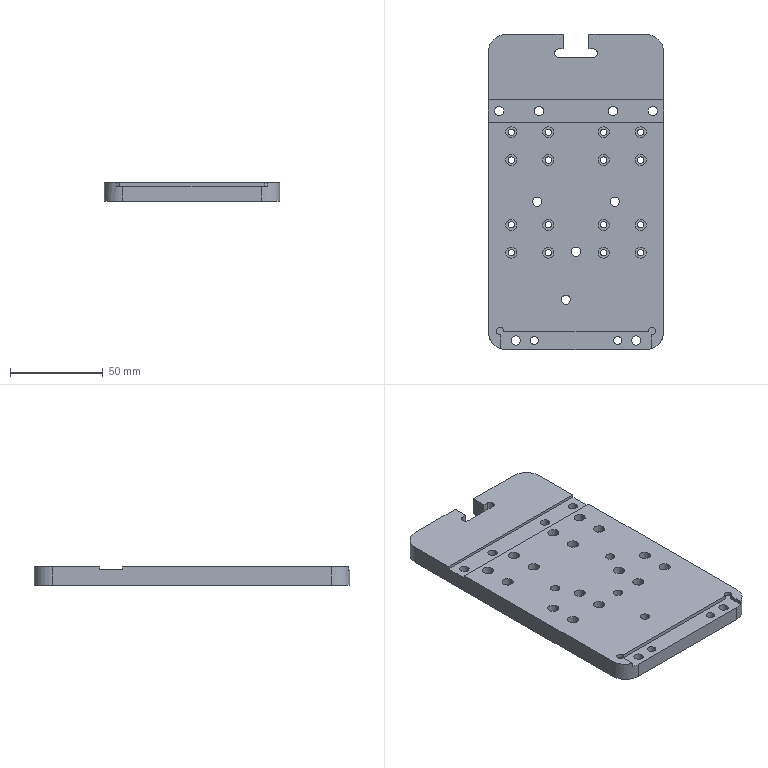Part | SolidWorks | features HoleWzd 8, ICE 8, Fillet 4, MoveFace 2, Cut 1, Extrusion 1, MirrorPattern 1 | 1 solid | 163 faces | box 95 x 170.5 x 10 mm | volume 143560 mm3 | cylinder 111 | plane 52 | commonest cylinder face diameters 3.4 x32 6 x32 5 x20 4 x15 4.4 x4 8 x4